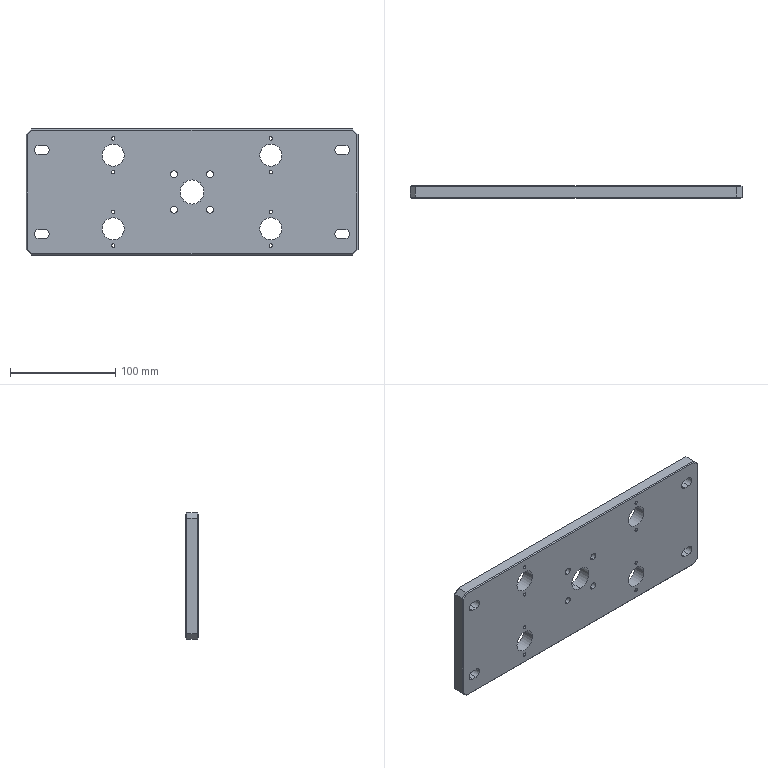Part | STEP file | BPSP-11-17 Unloading Linear Bearing Mounting Plate_Default | 1 solid | 88 faces | box 316 x 12 x 120 mm | volume 422737 mm3 | cylinder 50 | plane 38 | commonest cylinder face diameters 3.3 x16 6.6 x8 9 x8 11 x8 21 x8 23 x2